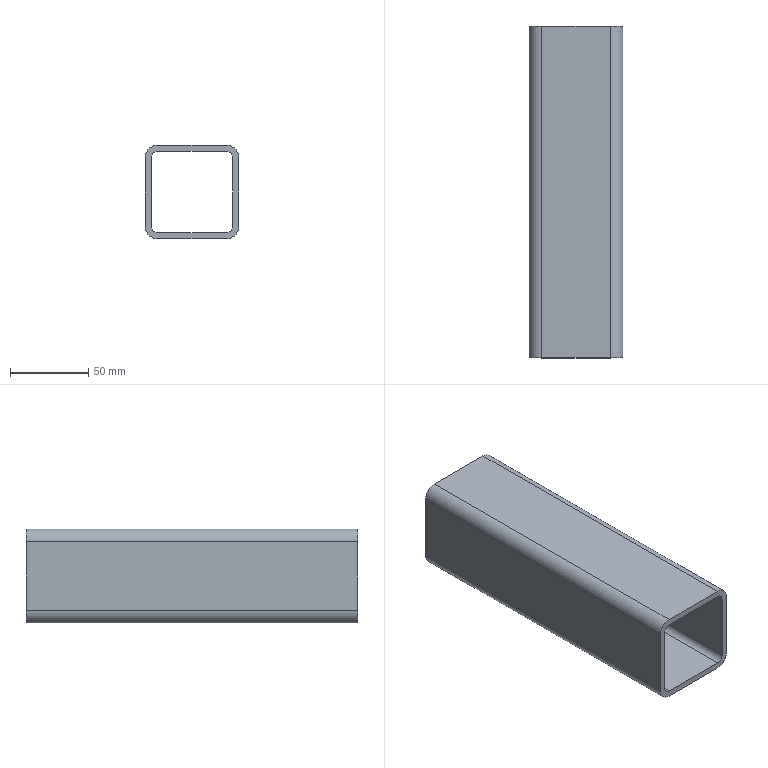Part | SolidWorks | features BaseBody 1 | 1 solid | 18 faces | box 60 x 212.456 x 60 mm | volume 181607 mm3 | plane 10 | cylinder 8 | commonest cylinder face diameters 8 x4 16 x4
STEP:
#1=CARTESIAN_POINT('',(26.,2212.,-28.));
#2=VERTEX_POINT('',#1);
#3=CARTESIAN_POINT('',(26.,2212.,-72.));
#4=VERTEX_POINT('',#3);
#5=CARTESIAN_POINT('',(26.,2212.,-28.));
#6=DIRECTION('',(0.,0.,-1.));
#7=VECTOR('',#6,1000.);
#8=LINE('',#5,#7);
#9=EDGE_CURVE('',#2,#4,#8,.T.);
#10=ORIENTED_EDGE('',*,*,#9,.T.);
#11=CARTESIAN_POINT('',(26.,1999.544,-72.));
#12=VERTEX_POINT('',#11);
#13=CARTESIAN_POINT('',(26.,2119.544,-72.));
#14=DIRECTION('',(0.,-1.,0.));
#15=VECTOR('',#14,1000.);
#16=LINE('',#13,#15);
#17=EDGE_CURVE('',#4,#12,#16,.T.);
#18=ORIENTED_EDGE('',*,*,#17,.T.);
#19=CARTESIAN_POINT('',(26.,1999.544,-28.));
#20=VERTEX_POINT('',#19);
#21=CARTESIAN_POINT('',(26.,1999.544,-28.));
#22=DIRECTION('',(0.,0.,1.));
#23=VECTOR('',#22,1000.);
#24=LINE('',#21,#23);
#25=EDGE_CURVE('',#12,#20,#24,.T.);
#26=ORIENTED_EDGE('',*,*,#25,.T.);
#27=CARTESIAN_POINT('',(26.,2119.544,-28.));
#28=DIRECTION('',(0.,1.,0.));
#29=VECTOR('',#28,1000.);
#30=LINE('',#27,#29);
#31=EDGE_CURVE('',#20,#2,#30,.T.);
#32=ORIENTED_EDGE('',*,*,#31,.T.);
#33=EDGE_LOOP('',(#10,#18,#26,#32));
#34=FACE_OUTER_BOUND('',#33,.T.);
#35=CARTESIAN_POINT('',(26.,2119.544,-28.));
#36=DIRECTION('',(-1.,0.,0.));
#37=DIRECTION('',(0.,0.,1.));
#38=AXIS2_PLACEMENT_3D('',#35,#36,#37);
#39=PLANE('',#38);
#40=ADVANCED_FACE('',(#34),#39,.T.);
#41=ORIENTED_EDGE('',*,*,#17,.F.);
#42=CARTESIAN_POINT('',(22.,2212.,-76.));
#43=VERTEX_POINT('',#42);
#44=CARTESIAN_POINT('',(22.,2212.,-72.));
#45=DIRECTION('',(0.,-1.,0.));
#46=DIRECTION('',(0.,0.,-1.));
#47=AXIS2_PLACEMENT_3D('',#44,#45,#46);
#48=CIRCLE('',#47,4.);
#49=EDGE_CURVE('',#43,#4,#48,.T.);
#50=ORIENTED_EDGE('',*,*,#49,.F.);
#51=CARTESIAN_POINT('',(22.,1999.544,-76.));
#52=VERTEX_POINT('',#51);
#53=CARTESIAN_POINT('',(22.,2119.544,-76.));
#54=DIRECTION('',(0.,1.,0.));
#55=VECTOR('',#54,1000.);
#56=LINE('',#53,#55);
#57=EDGE_CURVE('',#52,#43,#56,.T.);
#58=ORIENTED_EDGE('',*,*,#57,.F.);
#59=CARTESIAN_POINT('',(22.,1999.544,-72.));
#60=DIRECTION('',(0.,1.,0.));
#61=DIRECTION('',(0.,0.,-1.));
#62=AXIS2_PLACEMENT_3D('',#59,#60,#61);
#63=CIRCLE('',#62,4.);
#64=EDGE_CURVE('',#12,#52,#63,.T.);
#65=ORIENTED_EDGE('',*,*,#64,.F.);
#66=EDGE_LOOP('',(#41,#50,#58,#65));
#67=FACE_OUTER_BOUND('',#66,.T.);
#68=CARTESIAN_POINT('',(22.,2119.544,-72.));
#69=DIRECTION('',(0.,-1.,0.));
#70=DIRECTION('',(0.,0.,-1.));
#71=AXIS2_PLACEMENT_3D('',#68,#69,#70);
#72=CYLINDRICAL_SURFACE('',#71,4.);
#73=ADVANCED_FACE('',(#67),#72,.F.);
#74=CARTESIAN_POINT('',(-22.,2212.,-76.));
#75=VERTEX_POINT('',#74);
#76=CARTESIAN_POINT('',(-26.,2212.,-72.));
#77=VERTEX_POINT('',#76);
#78=CARTESIAN_POINT('',(-22.,2212.,-72.));
#79=DIRECTION('',(0.,1.,0.));
#80=DIRECTION('',(0.,0.,-1.));
#81=AXIS2_PLACEMENT_3D('',#78,#79,#80);
#82=CIRCLE('',#81,4.);
#83=EDGE_CURVE('',#75,#77,#82,.T.);
#84=ORIENTED_EDGE('',*,*,#83,.F.);
#85=CARTESIAN_POINT('',(22.,2212.,-76.));
#86=DIRECTION('',(-1.,0.,0.));
#87=VECTOR('',#86,1000.);
#88=LINE('',#85,#87);
#89=EDGE_CURVE('',#43,#75,#88,.T.);
#90=ORIENTED_EDGE('',*,*,#89,.F.);
#91=ORIENTED_EDGE('',*,*,#49,.T.);
#92=ORIENTED_EDGE('',*,*,#9,.F.);
#93=CARTESIAN_POINT('',(22.,2212.,-24.));
#94=VERTEX_POINT('',#93);
#95=CARTESIAN_POINT('',(22.,2212.,-28.));
#96=DIRECTION('',(0.,1.,0.));
#97=DIRECTION('',(0.,0.,-1.));
#98=AXIS2_PLACEMENT_3D('',#95,#96,#97);
#99=CIRCLE('',#98,4.);
#100=EDGE_CURVE('',#94,#2,#99,.T.);
#101=ORIENTED_EDGE('',*,*,#100,.F.);
#102=CARTESIAN_POINT('',(-22.,2212.,-24.));
#103=VERTEX_POINT('',#102);
#104=CARTESIAN_POINT('',(22.,2212.,-24.));
#105=DIRECTION('',(1.,0.,0.));
#106=VECTOR('',#105,1000.);
#107=LINE('',#104,#106);
#108=EDGE_CURVE('',#103,#94,#107,.T.);
#109=ORIENTED_EDGE('',*,*,#108,.F.);
#110=CARTESIAN_POINT('',(-26.,2212.,-28.));
#111=VERTEX_POINT('',#110);
#112=CARTESIAN_POINT('',(-22.,2212.,-28.));
#113=DIRECTION('',(0.,1.,0.));
#114=DIRECTION('',(0.,0.,-1.));
#115=AXIS2_PLACEMENT_3D('',#112,#113,#114);
#116=CIRCLE('',#115,4.);
#117=EDGE_CURVE('',#111,#103,#116,.T.);
#118=ORIENTED_EDGE('',*,*,#117,.F.);
#119=CARTESIAN_POINT('',(-26.,2212.,-1550.));
#120=DIRECTION('',(0.,0.,1.));
#121=VECTOR('',#120,1000.);
#122=LINE('',#119,#121);
#123=EDGE_CURVE('',#77,#111,#122,.T.);
#124=ORIENTED_EDGE('',*,*,#123,.F.);
#125=EDGE_LOOP('',(#84,#90,#91,#92,#101,#109,#118,#124));
#126=FACE_BOUND('',#125,.T.);
#127=CARTESIAN_POINT('',(-30.,2212.,-28.));
#128=VERTEX_POINT('',#127);
#129=CARTESIAN_POINT('',(-30.,2212.,-72.));
#130=VERTEX_POINT('',#129);
#131=CARTESIAN_POINT('',(-30.,2212.,-1550.));
#132=DIRECTION('',(0.,0.,-1.));
#133=VECTOR('',#132,1000.);
#134=LINE('',#131,#133);
#135=EDGE_CURVE('',#128,#130,#134,.T.);
#136=ORIENTED_EDGE('',*,*,#135,.F.);
#137=CARTESIAN_POINT('',(-22.,2212.,-20.));
#138=VERTEX_POINT('',#137);
#139=CARTESIAN_POINT('',(-22.,2212.,-28.));
#140=DIRECTION('',(0.,-1.,0.));
#141=DIRECTION('',(0.,0.,-1.));
#142=AXIS2_PLACEMENT_3D('',#139,#140,#141);
#143=CIRCLE('',#142,8.);
#144=EDGE_CURVE('',#138,#128,#143,.T.);
#145=ORIENTED_EDGE('',*,*,#144,.F.);
#146=CARTESIAN_POINT('',(22.,2212.,-20.));
#147=VERTEX_POINT('',#146);
#148=CARTESIAN_POINT('',(22.,2212.,-20.));
#149=DIRECTION('',(-1.,0.,0.));
#150=VECTOR('',#149,1000.);
#151=LINE('',#148,#150);
#152=EDGE_CURVE('',#147,#138,#151,.T.);
#153=ORIENTED_EDGE('',*,*,#152,.F.);
#154=CARTESIAN_POINT('',(30.,2212.,-28.));
#155=VERTEX_POINT('',#154);
#156=CARTESIAN_POINT('',(22.,2212.,-28.));
#157=DIRECTION('',(0.,-1.,0.));
#158=DIRECTION('',(0.,0.,-1.));
#159=AXIS2_PLACEMENT_3D('',#156,#157,#158);
#160=CIRCLE('',#159,8.);
#161=EDGE_CURVE('',#155,#147,#160,.T.);
#162=ORIENTED_EDGE('',*,*,#161,.F.);
#163=CARTESIAN_POINT('',(30.,2212.,-72.));
#164=VERTEX_POINT('',#163);
#165=CARTESIAN_POINT('',(30.,2212.,-1550.));
#166=DIRECTION('',(0.,0.,1.));
#167=VECTOR('',#166,1000.);
#168=LINE('',#165,#167);
#169=EDGE_CURVE('',#164,#155,#168,.T.);
#170=ORIENTED_EDGE('',*,*,#169,.F.);
#171=CARTESIAN_POINT('',(22.,2212.,-80.));
#172=VERTEX_POINT('',#171);
#173=CARTESIAN_POINT('',(22.,2212.,-72.));
#174=DIRECTION('',(0.,-1.,0.));
#175=DIRECTION('',(0.,0.,-1.));
#176=AXIS2_PLACEMENT_3D('',#173,#174,#175);
#177=CIRCLE('',#176,8.);
#178=EDGE_CURVE('',#172,#164,#177,.T.);
#179=ORIENTED_EDGE('',*,*,#178,.F.);
#180=CARTESIAN_POINT('',(-22.,2212.,-80.));
#181=VERTEX_POINT('',#180);
#182=CARTESIAN_POINT('',(22.,2212.,-80.));
#183=DIRECTION('',(1.,0.,0.));
#184=VECTOR('',#183,1000.);
#185=LINE('',#182,#184);
#186=EDGE_CURVE('',#181,#172,#185,.T.);
#187=ORIENTED_EDGE('',*,*,#186,.F.);
#188=CARTESIAN_POINT('',(-22.,2212.,-72.));
#189=DIRECTION('',(0.,-1.,0.));
#190=DIRECTION('',(0.,0.,-1.));
#191=AXIS2_PLACEMENT_3D('',#188,#189,#190);
#192=CIRCLE('',#191,8.);
#193=EDGE_CURVE('',#130,#181,#192,.T.);
#194=ORIENTED_EDGE('',*,*,#193,.F.);
#195=EDGE_LOOP('',(#136,#145,#153,#162,#170,#179,#187,#194));
#196=FACE_OUTER_BOUND('',#195,.T.);
#197=CARTESIAN_POINT('',(22.,2212.,-1550.));
#198=DIRECTION('',(0.,-1.,0.));
#199=DIRECTION('',(0.,0.,-1.));
#200=AXIS2_PLACEMENT_3D('',#197,#198,#199);
#201=PLANE('',#200);
#202=ADVANCED_FACE('',(#126,#196),#201,.F.);
#203=CARTESIAN_POINT('',(22.,1999.544,-24.));
#204=VERTEX_POINT('',#203);
#205=CARTESIAN_POINT('',(22.,2119.544,-24.));
#206=DIRECTION('',(0.,-1.,0.));
#207=VECTOR('',#206,1000.);
#208=LINE('',#205,#207);
#209=EDGE_CURVE('',#94,#204,#208,.T.);
#210=ORIENTED_EDGE('',*,*,#209,.F.);
#211=ORIENTED_EDGE('',*,*,#100,.T.);
#212=ORIENTED_EDGE('',*,*,#31,.F.);
#213=CARTESIAN_POINT('',(22.,1999.544,-28.));
#214=DIRECTION('',(0.,1.,0.));
#215=DIRECTION('',(0.,0.,-1.));
#216=AXIS2_PLACEMENT_3D('',#213,#214,#215);
#217=CIRCLE('',#216,4.);
#218=EDGE_CURVE('',#204,#20,#217,.T.);
#219=ORIENTED_EDGE('',*,*,#218,.F.);
#220=EDGE_LOOP('',(#210,#211,#212,#219));
#221=FACE_OUTER_BOUND('',#220,.T.);
#222=CARTESIAN_POINT('',(22.,2119.544,-28.));
#223=DIRECTION('',(0.,-1.,0.));
#224=DIRECTION('',(0.,0.,-1.));
#225=AXIS2_PLACEMENT_3D('',#222,#223,#224);
#226=CYLINDRICAL_SURFACE('',#225,4.);
#227=ADVANCED_FACE('',(#221),#226,.F.);
#228=CARTESIAN_POINT('',(-26.,1999.544,-28.));
#229=VERTEX_POINT('',#228);
#230=CARTESIAN_POINT('',(-22.,1999.544,-24.));
#231=VERTEX_POINT('',#230);
#232=CARTESIAN_POINT('',(-22.,1999.544,-28.));
#233=DIRECTION('',(0.,1.,0.));
#234=DIRECTION('',(0.,0.,-1.));
#235=AXIS2_PLACEMENT_3D('',#232,#233,#234);
#236=CIRCLE('',#235,4.);
#237=EDGE_CURVE('',#229,#231,#236,.T.);
#238=ORIENTED_EDGE('',*,*,#237,.T.);
#239=CARTESIAN_POINT('',(-22.,1999.544,-24.));
#240=DIRECTION('',(1.,0.,0.));
#241=VECTOR('',#240,1000.);
#242=LINE('',#239,#241);
#243=EDGE_CURVE('',#231,#204,#242,.T.);
#244=ORIENTED_EDGE('',*,*,#243,.T.);
#245=ORIENTED_EDGE('',*,*,#218,.T.);
#246=ORIENTED_EDGE('',*,*,#25,.F.);
#247=ORIENTED_EDGE('',*,*,#64,.T.);
#248=CARTESIAN_POINT('',(-22.,1999.544,-76.));
#249=VERTEX_POINT('',#248);
#250=CARTESIAN_POINT('',(-22.,1999.544,-76.));
#251=DIRECTION('',(-1.,0.,0.));
#252=VECTOR('',#251,1000.);
#253=LINE('',#250,#252);
#254=EDGE_CURVE('',#52,#249,#253,.T.);
#255=ORIENTED_EDGE('',*,*,#254,.T.);
#256=CARTESIAN_POINT('',(-26.,1999.544,-72.));
#257=VERTEX_POINT('',#256);
#258=CARTESIAN_POINT('',(-22.,1999.544,-72.));
#259=DIRECTION('',(0.,1.,0.));
#260=DIRECTION('',(0.,0.,-1.));
#261=AXIS2_PLACEMENT_3D('',#258,#259,#260);
#262=CIRCLE('',#261,4.);
#263=EDGE_CURVE('',#249,#257,#262,.T.);
#264=ORIENTED_EDGE('',*,*,#263,.T.);
#265=CARTESIAN_POINT('',(-26.,1999.544,-50.));
#266=DIRECTION('',(0.,0.,1.));
#267=VECTOR('',#266,1000.);
#268=LINE('',#265,#267);
#269=EDGE_CURVE('',#257,#229,#268,.T.);
#270=ORIENTED_EDGE('',*,*,#269,.T.);
#271=EDGE_LOOP('',(#238,#244,#245,#246,#247,#255,#264,#270));
#272=FACE_BOUND('',#271,.T.);
#273=CARTESIAN_POINT('',(22.,1999.544,-20.));
#274=VERTEX_POINT('',#273);
#275=CARTESIAN_POINT('',(-22.,1999.544,-20.));
#276=VERTEX_POINT('',#275);
#277=CARTESIAN_POINT('',(-22.,1999.544,-20.));
#278=DIRECTION('',(-1.,0.,0.));
#279=VECTOR('',#278,1000.);
#280=LINE('',#277,#279);
#281=EDGE_CURVE('',#274,#276,#280,.T.);
#282=ORIENTED_EDGE('',*,*,#281,.T.);
#283=CARTESIAN_POINT('',(-30.,1999.544,-28.));
#284=VERTEX_POINT('',#283);
#285=CARTESIAN_POINT('',(-22.,1999.544,-28.));
#286=DIRECTION('',(0.,-1.,0.));
#287=DIRECTION('',(0.,0.,-1.));
#288=AXIS2_PLACEMENT_3D('',#285,#286,#287);
#289=CIRCLE('',#288,8.);
#290=EDGE_CURVE('',#276,#284,#289,.T.);
#291=ORIENTED_EDGE('',*,*,#290,.T.);
#292=CARTESIAN_POINT('',(-30.,1999.544,-72.));
#293=VERTEX_POINT('',#292);
#294=CARTESIAN_POINT('',(-30.,1999.544,-50.));
#295=DIRECTION('',(0.,0.,-1.));
#296=VECTOR('',#295,1000.);
#297=LINE('',#294,#296);
#298=EDGE_CURVE('',#284,#293,#297,.T.);
#299=ORIENTED_EDGE('',*,*,#298,.T.);
#300=CARTESIAN_POINT('',(-22.,1999.544,-80.));
#301=VERTEX_POINT('',#300);
#302=CARTESIAN_POINT('',(-22.,1999.544,-72.));
#303=DIRECTION('',(0.,-1.,0.));
#304=DIRECTION('',(0.,0.,-1.));
#305=AXIS2_PLACEMENT_3D('',#302,#303,#304);
#306=CIRCLE('',#305,8.);
#307=EDGE_CURVE('',#293,#301,#306,.T.);
#308=ORIENTED_EDGE('',*,*,#307,.T.);
#309=CARTESIAN_POINT('',(22.,1999.544,-80.));
#310=VERTEX_POINT('',#309);
#311=CARTESIAN_POINT('',(-22.,1999.544,-80.));
#312=DIRECTION('',(1.,0.,0.));
#313=VECTOR('',#312,1000.);
#314=LINE('',#311,#313);
#315=EDGE_CURVE('',#301,#310,#314,.T.);
#316=ORIENTED_EDGE('',*,*,#315,.T.);
#317=CARTESIAN_POINT('',(30.,1999.544,-72.));
#318=VERTEX_POINT('',#317);
#319=CARTESIAN_POINT('',(22.,1999.544,-72.));
#320=DIRECTION('',(0.,-1.,0.));
#321=DIRECTION('',(0.,0.,-1.));
#322=AXIS2_PLACEMENT_3D('',#319,#320,#321);
#323=CIRCLE('',#322,8.);
#324=EDGE_CURVE('',#310,#318,#323,.T.);
#325=ORIENTED_EDGE('',*,*,#324,.T.);
#326=CARTESIAN_POINT('',(30.,1999.544,-28.));
#327=VERTEX_POINT('',#326);
#328=CARTESIAN_POINT('',(30.,1999.544,-50.));
#329=DIRECTION('',(0.,0.,1.));
#330=VECTOR('',#329,1000.);
#331=LINE('',#328,#330);
#332=EDGE_CURVE('',#318,#327,#331,.T.);
#333=ORIENTED_EDGE('',*,*,#332,.T.);
#334=CARTESIAN_POINT('',(22.,1999.544,-28.));
#335=DIRECTION('',(0.,-1.,0.));
#336=DIRECTION('',(0.,0.,-1.));
#337=AXIS2_PLACEMENT_3D('',#334,#335,#336);
#338=CIRCLE('',#337,8.);
#339=EDGE_CURVE('',#327,#274,#338,.T.);
#340=ORIENTED_EDGE('',*,*,#339,.T.);
#341=EDGE_LOOP('',(#282,#291,#299,#308,#316,#325,#333,#340));
#342=FACE_OUTER_BOUND('',#341,.T.);
#343=CARTESIAN_POINT('',(-22.,1999.544,-50.));
#344=DIRECTION('',(0.,-1.,0.));
#345=DIRECTION('',(0.,0.,-1.));
#346=AXIS2_PLACEMENT_3D('',#343,#344,#345);
#347=PLANE('',#346);
#348=ADVANCED_FACE('',(#272,#342),#347,.T.);
#349=ORIENTED_EDGE('',*,*,#89,.T.);
#350=CARTESIAN_POINT('',(-22.,2119.544,-76.));
#351=DIRECTION('',(0.,-1.,0.));
#352=VECTOR('',#351,1000.);
#353=LINE('',#350,#352);
#354=EDGE_CURVE('',#75,#249,#353,.T.);
#355=ORIENTED_EDGE('',*,*,#354,.T.);
#356=ORIENTED_EDGE('',*,*,#254,.F.);
#357=ORIENTED_EDGE('',*,*,#57,.T.);
#358=EDGE_LOOP('',(#349,#355,#356,#357));
#359=FACE_OUTER_BOUND('',#358,.T.);
#360=CARTESIAN_POINT('',(-22.,2119.544,-76.));
#361=DIRECTION('',(0.,0.,1.));
#362=DIRECTION('',(1.,0.,0.));
#363=AXIS2_PLACEMENT_3D('',#360,#361,#362);
#364=PLANE('',#363);
#365=ADVANCED_FACE('',(#359),#364,.T.);
#366=ORIENTED_EDGE('',*,*,#123,.T.);
#367=CARTESIAN_POINT('',(-26.,2119.544,-28.));
#368=DIRECTION('',(0.,-1.,0.));
#369=VECTOR('',#368,1000.);
#370=LINE('',#367,#369);
#371=EDGE_CURVE('',#111,#229,#370,.T.);
#372=ORIENTED_EDGE('',*,*,#371,.T.);
#373=ORIENTED_EDGE('',*,*,#269,.F.);
#374=CARTESIAN_POINT('',(-26.,2119.544,-72.));
#375=DIRECTION('',(0.,1.,0.));
#376=VECTOR('',#375,1000.);
#377=LINE('',#374,#376);
#378=EDGE_CURVE('',#257,#77,#377,.T.);
#379=ORIENTED_EDGE('',*,*,#378,.T.);
#380=EDGE_LOOP('',(#366,#372,#373,#379));
#381=FACE_OUTER_BOUND('',#380,.T.);
#382=CARTESIAN_POINT('',(-26.,2119.544,-72.));
#383=DIRECTION('',(1.,0.,0.));
#384=DIRECTION('',(0.,0.,-1.));
#385=AXIS2_PLACEMENT_3D('',#382,#383,#384);
#386=PLANE('',#385);
#387=ADVANCED_FACE('',(#381),#386,.T.);
#388=ORIENTED_EDGE('',*,*,#354,.F.);
#389=ORIENTED_EDGE('',*,*,#83,.T.);
#390=ORIENTED_EDGE('',*,*,#378,.F.);
#391=ORIENTED_EDGE('',*,*,#263,.F.);
#392=EDGE_LOOP('',(#388,#389,#390,#391));
#393=FACE_OUTER_BOUND('',#392,.T.);
#394=CARTESIAN_POINT('',(-22.,2119.544,-72.));
#395=DIRECTION('',(0.,-1.,0.));
#396=DIRECTION('',(0.,0.,-1.));
#397=AXIS2_PLACEMENT_3D('',#394,#395,#396);
#398=CYLINDRICAL_SURFACE('',#397,4.);
#399=ADVANCED_FACE('',(#393),#398,.F.);
#400=ORIENTED_EDGE('',*,*,#108,.T.);
#401=ORIENTED_EDGE('',*,*,#209,.T.);
#402=ORIENTED_EDGE('',*,*,#243,.F.);
#403=CARTESIAN_POINT('',(-22.,2119.544,-24.));
#404=DIRECTION('',(0.,1.,0.));
#405=VECTOR('',#404,1000.);
#406=LINE('',#403,#405);
#407=EDGE_CURVE('',#231,#103,#406,.T.);
#408=ORIENTED_EDGE('',*,*,#407,.T.);
#409=EDGE_LOOP('',(#400,#401,#402,#408));
#410=FACE_OUTER_BOUND('',#409,.T.);
#411=CARTESIAN_POINT('',(22.,2119.544,-24.));
#412=DIRECTION('',(0.,0.,-1.));
#413=DIRECTION('',(-1.,0.,0.));
#414=AXIS2_PLACEMENT_3D('',#411,#412,#413);
#415=PLANE('',#414);
#416=ADVANCED_FACE('',(#410),#415,.T.);
#417=ORIENTED_EDGE('',*,*,#371,.F.);
#418=ORIENTED_EDGE('',*,*,#117,.T.);
#419=ORIENTED_EDGE('',*,*,#407,.F.);
#420=ORIENTED_EDGE('',*,*,#237,.F.);
#421=EDGE_LOOP('',(#417,#418,#419,#420));
#422=FACE_OUTER_BOUND('',#421,.T.);
#423=CARTESIAN_POINT('',(-22.,2119.544,-28.));
#424=DIRECTION('',(0.,-1.,0.));
#425=DIRECTION('',(0.,0.,-1.));
#426=AXIS2_PLACEMENT_3D('',#423,#424,#425);
#427=CYLINDRICAL_SURFACE('',#426,4.);
#428=ADVANCED_FACE('',(#422),#427,.F.);
#429=CARTESIAN_POINT('',(-22.,2119.544,-80.));
#430=DIRECTION('',(0.,-1.,0.));
#431=VECTOR('',#430,1000.);
#432=LINE('',#429,#431);
#433=EDGE_CURVE('',#181,#301,#432,.T.);
#434=ORIENTED_EDGE('',*,*,#433,.T.);
#435=ORIENTED_EDGE('',*,*,#307,.F.);
#436=CARTESIAN_POINT('',(-30.,2119.544,-72.));
#437=DIRECTION('',(0.,1.,0.));
#438=VECTOR('',#437,1000.);
#439=LINE('',#436,#438);
#440=EDGE_CURVE('',#293,#130,#439,.T.);
#441=ORIENTED_EDGE('',*,*,#440,.T.);
#442=ORIENTED_EDGE('',*,*,#193,.T.);
#443=EDGE_LOOP('',(#434,#435,#441,#442));
#444=FACE_OUTER_BOUND('',#443,.T.);
#445=CARTESIAN_POINT('',(-22.,2119.544,-72.));
#446=DIRECTION('',(0.,-1.,0.));
#447=DIRECTION('',(0.,0.,-1.));
#448=AXIS2_PLACEMENT_3D('',#445,#446,#447);
#449=CYLINDRICAL_SURFACE('',#448,8.);
#450=ADVANCED_FACE('',(#444),#449,.T.);
#451=ORIENTED_EDGE('',*,*,#135,.T.);
#452=ORIENTED_EDGE('',*,*,#440,.F.);
#453=ORIENTED_EDGE('',*,*,#298,.F.);
#454=CARTESIAN_POINT('',(-30.,2119.544,-28.));
#455=DIRECTION('',(0.,-1.,0.));
#456=VECTOR('',#455,1000.);
#457=LINE('',#454,#456);
#458=EDGE_CURVE('',#128,#284,#457,.T.);
#459=ORIENTED_EDGE('',*,*,#458,.F.);
#460=EDGE_LOOP('',(#451,#452,#453,#459));
#461=FACE_OUTER_BOUND('',#460,.T.);
#462=CARTESIAN_POINT('',(-30.,2119.544,-72.));
#463=DIRECTION('',(1.,0.,0.));
#464=DIRECTION('',(0.,0.,-1.));
#465=AXIS2_PLACEMENT_3D('',#462,#463,#464);
#466=PLANE('',#465);
#467=ADVANCED_FACE('',(#461),#466,.F.);
#468=ORIENTED_EDGE('',*,*,#458,.T.);
#469=ORIENTED_EDGE('',*,*,#290,.F.);
#470=CARTESIAN_POINT('',(-22.,2119.544,-20.));
#471=DIRECTION('',(0.,1.,0.));
#472=VECTOR('',#471,1000.);
#473=LINE('',#470,#472);
#474=EDGE_CURVE('',#276,#138,#473,.T.);
#475=ORIENTED_EDGE('',*,*,#474,.T.);
#476=ORIENTED_EDGE('',*,*,#144,.T.);
#477=EDGE_LOOP('',(#468,#469,#475,#476));
#478=FACE_OUTER_BOUND('',#477,.T.);
#479=CARTESIAN_POINT('',(-22.,2119.544,-28.));
#480=DIRECTION('',(0.,-1.,0.));
#481=DIRECTION('',(0.,0.,-1.));
#482=AXIS2_PLACEMENT_3D('',#479,#480,#481);
#483=CYLINDRICAL_SURFACE('',#482,8.);
#484=ADVANCED_FACE('',(#478),#483,.T.);
#485=ORIENTED_EDGE('',*,*,#152,.T.);
#486=ORIENTED_EDGE('',*,*,#474,.F.);
#487=ORIENTED_EDGE('',*,*,#281,.F.);
#488=CARTESIAN_POINT('',(22.,2119.544,-20.));
#489=DIRECTION('',(0.,-1.,0.));
#490=VECTOR('',#489,1000.);
#491=LINE('',#488,#490);
#492=EDGE_CURVE('',#147,#274,#491,.T.);
#493=ORIENTED_EDGE('',*,*,#492,.F.);
#494=EDGE_LOOP('',(#485,#486,#487,#493));
#495=FACE_OUTER_BOUND('',#494,.T.);
#496=CARTESIAN_POINT('',(22.,2119.544,-20.));
#497=DIRECTION('',(0.,0.,-1.));
#498=DIRECTION('',(-1.,0.,0.));
#499=AXIS2_PLACEMENT_3D('',#496,#497,#498);
#500=PLANE('',#499);
#501=ADVANCED_FACE('',(#495),#500,.F.);
#502=ORIENTED_EDGE('',*,*,#492,.T.);
#503=ORIENTED_EDGE('',*,*,#339,.F.);
#504=CARTESIAN_POINT('',(30.,2119.544,-28.));
#505=DIRECTION('',(0.,1.,0.));
#506=VECTOR('',#505,1000.);
#507=LINE('',#504,#506);
#508=EDGE_CURVE('',#327,#155,#507,.T.);
#509=ORIENTED_EDGE('',*,*,#508,.T.);
#510=ORIENTED_EDGE('',*,*,#161,.T.);
#511=EDGE_LOOP('',(#502,#503,#509,#510));
#512=FACE_OUTER_BOUND('',#511,.T.);
#513=CARTESIAN_POINT('',(22.,2119.544,-28.));
#514=DIRECTION('',(0.,-1.,0.));
#515=DIRECTION('',(0.,0.,-1.));
#516=AXIS2_PLACEMENT_3D('',#513,#514,#515);
#517=CYLINDRICAL_SURFACE('',#516,8.);
#518=ADVANCED_FACE('',(#512),#517,.T.);
#519=ORIENTED_EDGE('',*,*,#169,.T.);
#520=ORIENTED_EDGE('',*,*,#508,.F.);
#521=ORIENTED_EDGE('',*,*,#332,.F.);
#522=CARTESIAN_POINT('',(30.,2119.544,-72.));
#523=DIRECTION('',(0.,-1.,0.));
#524=VECTOR('',#523,1000.);
#525=LINE('',#522,#524);
#526=EDGE_CURVE('',#164,#318,#525,.T.);
#527=ORIENTED_EDGE('',*,*,#526,.F.);
#528=EDGE_LOOP('',(#519,#520,#521,#527));
#529=FACE_OUTER_BOUND('',#528,.T.);
#530=CARTESIAN_POINT('',(30.,2119.544,-28.));
#531=DIRECTION('',(-1.,0.,0.));
#532=DIRECTION('',(0.,0.,1.));
#533=AXIS2_PLACEMENT_3D('',#530,#531,#532);
#534=PLANE('',#533);
#535=ADVANCED_FACE('',(#529),#534,.F.);
#536=ORIENTED_EDGE('',*,*,#526,.T.);
#537=ORIENTED_EDGE('',*,*,#324,.F.);
#538=CARTESIAN_POINT('',(22.,2119.544,-80.));
#539=DIRECTION('',(0.,1.,0.));
#540=VECTOR('',#539,1000.);
#541=LINE('',#538,#540);
#542=EDGE_CURVE('',#310,#172,#541,.T.);
#543=ORIENTED_EDGE('',*,*,#542,.T.);
#544=ORIENTED_EDGE('',*,*,#178,.T.);
#545=EDGE_LOOP('',(#536,#537,#543,#544));
#546=FACE_OUTER_BOUND('',#545,.T.);
#547=CARTESIAN_POINT('',(22.,2119.544,-72.));
#548=DIRECTION('',(0.,-1.,0.));
#549=DIRECTION('',(0.,0.,-1.));
#550=AXIS2_PLACEMENT_3D('',#547,#548,#549);
#551=CYLINDRICAL_SURFACE('',#550,8.);
#552=ADVANCED_FACE('',(#546),#551,.T.);
#553=ORIENTED_EDGE('',*,*,#186,.T.);
#554=ORIENTED_EDGE('',*,*,#542,.F.);
#555=ORIENTED_EDGE('',*,*,#315,.F.);
#556=ORIENTED_EDGE('',*,*,#433,.F.);
#557=EDGE_LOOP('',(#553,#554,#555,#556));
#558=FACE_OUTER_BOUND('',#557,.T.);
#559=CARTESIAN_POINT('',(-22.,2119.544,-80.));
#560=DIRECTION('',(0.,0.,1.));
#561=DIRECTION('',(1.,0.,0.));
#562=AXIS2_PLACEMENT_3D('',#559,#560,#561);
#563=PLANE('',#562);
#564=ADVANCED_FACE('',(#558),#563,.F.);
#565=CLOSED_SHELL('',(#40,#73,#202,#227,#348,#365,#387,#399,#416,#428,#450,#467,#484,#501,#518,#535,#552,#564));
#566=MANIFOLD_SOLID_BREP('',#565);
#567=CARTESIAN_POINT('',(0.,0.,0.));
#568=DIRECTION('',(0.,0.,1.));
#569=DIRECTION('',(1.,0.,0.));
#570=AXIS2_PLACEMENT_3D('',#567,#568,#569);
#571=(LENGTH_UNIT()NAMED_UNIT(*)SI_UNIT(.MILLI.,.METRE.));
#572=UNCERTAINTY_MEASURE_WITH_UNIT(LENGTH_MEASURE(0.00001),#571,'','');
#573=(NAMED_UNIT(*)PLANE_ANGLE_UNIT()SI_UNIT($,.RADIAN.));
#574=(NAMED_UNIT(*)SI_UNIT($,.STERADIAN.)SOLID_ANGLE_UNIT());
#575=(GEOMETRIC_REPRESENTATION_CONTEXT(3)GLOBAL_UNCERTAINTY_ASSIGNED_CONTEXT((#572))GLOBAL_UNIT_ASSIGNED_CONTEXT((#571,#573,#574))REPRESENTATION_CONTEXT('',''));
#576=ADVANCED_BREP_SHAPE_REPRESENTATION('',(#566,#570),#575);